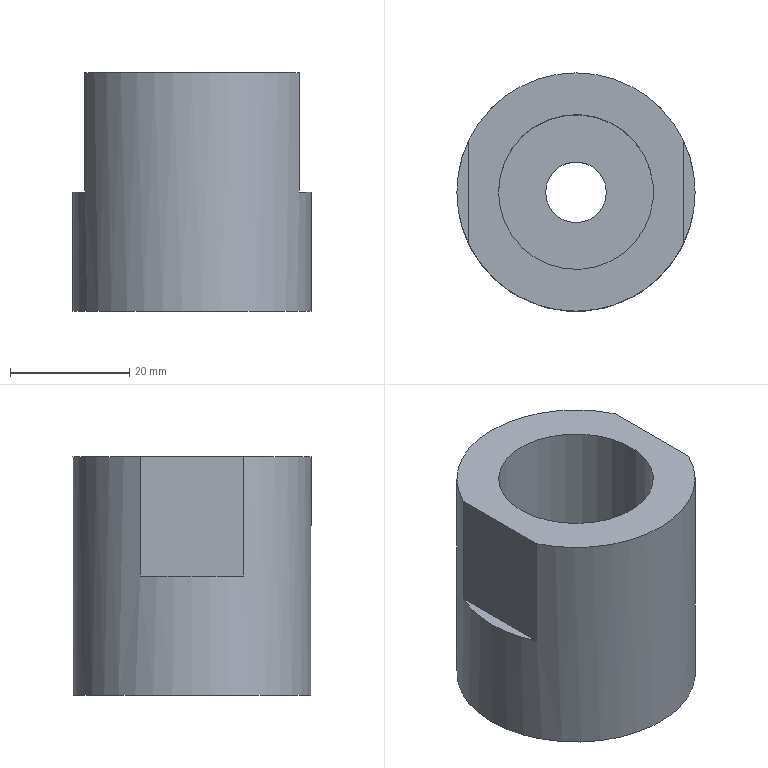Part | NX | features clamp stopper 2 | 1 solid | 10 faces | box 40 x 40 x 40 mm | volume 32581 mm3 | plane 7 | cylinder 3 | commonest cylinder face diameters 10.2 x1 26 x1 40 x1
STEP:
#1=CARTESIAN_POINT('',(-13.,0.,10.));
#2=VERTEX_POINT('',#1);
#3=CARTESIAN_POINT('',(0.,0.,10.));
#4=DIRECTION('',(0.,0.,-1.));
#5=DIRECTION('',(-1.,0.,0.));
#6=AXIS2_PLACEMENT_3D('',#3,#4,#5);
#7=CIRCLE('',#6,13.);
#8=EDGE_CURVE('',#2,#2,#7,.F.);
#9=ORIENTED_EDGE('',*,*,#8,.T.);
#10=EDGE_LOOP('',(#9));
#11=FACE_BOUND('',#10,.T.);
#12=CARTESIAN_POINT('',(5.1,0.,10.));
#13=VERTEX_POINT('',#12);
#14=CARTESIAN_POINT('',(0.,0.,10.));
#15=DIRECTION('',(0.,0.,1.));
#16=DIRECTION('',(1.,0.,0.));
#17=AXIS2_PLACEMENT_3D('',#14,#15,#16);
#18=CIRCLE('',#17,5.1);
#19=EDGE_CURVE('',#13,#13,#18,.F.);
#20=ORIENTED_EDGE('',*,*,#19,.T.);
#21=EDGE_LOOP('',(#20));
#22=FACE_BOUND('',#21,.T.);
#23=CARTESIAN_POINT('',(0.,0.,10.));
#24=DIRECTION('',(0.,0.,-1.));
#25=DIRECTION('',(-1.,0.,0.));
#26=AXIS2_PLACEMENT_3D('',#23,#24,#25);
#27=PLANE('',#26);
#28=ADVANCED_FACE('',(#11,#22),#27,.F.);
#29=ORIENTED_EDGE('',*,*,#8,.F.);
#30=EDGE_LOOP('',(#29));
#31=FACE_BOUND('',#30,.T.);
#32=CARTESIAN_POINT('',(-13.,0.,40.));
#33=VERTEX_POINT('',#32);
#34=CARTESIAN_POINT('',(0.,0.,40.));
#35=DIRECTION('',(0.,0.,-1.));
#36=DIRECTION('',(-1.,0.,0.));
#37=AXIS2_PLACEMENT_3D('',#34,#35,#36);
#38=CIRCLE('',#37,13.);
#39=EDGE_CURVE('',#33,#33,#38,.T.);
#40=ORIENTED_EDGE('',*,*,#39,.F.);
#41=EDGE_LOOP('',(#40));
#42=FACE_BOUND('',#41,.T.);
#43=CARTESIAN_POINT('',(0.,0.,40.));
#44=DIRECTION('',(0.,0.,-1.));
#45=DIRECTION('',(-1.,0.,0.));
#46=AXIS2_PLACEMENT_3D('',#43,#44,#45);
#47=CYLINDRICAL_SURFACE('',#46,13.);
#48=ADVANCED_FACE('',(#31,#42),#47,.F.);
#49=CARTESIAN_POINT('',(5.1,0.,0.));
#50=VERTEX_POINT('',#49);
#51=CARTESIAN_POINT('',(0.,0.,0.));
#52=DIRECTION('',(0.,0.,1.));
#53=DIRECTION('',(1.,0.,0.));
#54=AXIS2_PLACEMENT_3D('',#51,#52,#53);
#55=CIRCLE('',#54,5.1);
#56=EDGE_CURVE('',#50,#50,#55,.F.);
#57=ORIENTED_EDGE('',*,*,#56,.T.);
#58=EDGE_LOOP('',(#57));
#59=FACE_BOUND('',#58,.T.);
#60=ORIENTED_EDGE('',*,*,#19,.F.);
#61=EDGE_LOOP('',(#60));
#62=FACE_BOUND('',#61,.T.);
#63=CARTESIAN_POINT('',(0.,0.,10.));
#64=DIRECTION('',(0.,0.,1.));
#65=DIRECTION('',(1.,0.,0.));
#66=AXIS2_PLACEMENT_3D('',#63,#64,#65);
#67=CYLINDRICAL_SURFACE('',#66,5.1);
#68=ADVANCED_FACE('',(#59,#62),#67,.F.);
#69=CARTESIAN_POINT('',(18.,8.718,20.));
#70=VERTEX_POINT('',#69);
#71=CARTESIAN_POINT('',(18.,-8.718,20.));
#72=VERTEX_POINT('',#71);
#73=CARTESIAN_POINT('',(0.,0.,20.));
#74=DIRECTION('',(0.,0.,-1.));
#75=DIRECTION('',(-1.,0.,0.));
#76=AXIS2_PLACEMENT_3D('',#73,#74,#75);
#77=CIRCLE('',#76,20.);
#78=EDGE_CURVE('',#70,#72,#77,.T.);
#79=ORIENTED_EDGE('',*,*,#78,.F.);
#80=CARTESIAN_POINT('',(18.,-20.,20.));
#81=DIRECTION('',(0.,1.,0.));
#82=VECTOR('',#81,1000.);
#83=LINE('',#80,#82);
#84=EDGE_CURVE('',#72,#70,#83,.T.);
#85=ORIENTED_EDGE('',*,*,#84,.F.);
#86=EDGE_LOOP('',(#79,#85));
#87=FACE_BOUND('',#86,.T.);
#88=CARTESIAN_POINT('',(0.,0.,20.));
#89=DIRECTION('',(0.,0.,1.));
#90=DIRECTION('',(1.,0.,0.));
#91=AXIS2_PLACEMENT_3D('',#88,#89,#90);
#92=PLANE('',#91);
#93=ADVANCED_FACE('',(#87),#92,.T.);
#94=CARTESIAN_POINT('',(18.,8.718,40.));
#95=VERTEX_POINT('',#94);
#96=CARTESIAN_POINT('',(18.,8.718,40.));
#97=DIRECTION('',(0.,0.,-1.));
#98=VECTOR('',#97,1000.);
#99=LINE('',#96,#98);
#100=EDGE_CURVE('',#95,#70,#99,.T.);
#101=ORIENTED_EDGE('',*,*,#100,.F.);
#102=CARTESIAN_POINT('',(18.,-8.718,40.));
#103=VERTEX_POINT('',#102);
#104=CARTESIAN_POINT('',(18.,0.,40.));
#105=DIRECTION('',(0.,1.,0.));
#106=VECTOR('',#105,1000.);
#107=LINE('',#104,#106);
#108=EDGE_CURVE('',#103,#95,#107,.T.);
#109=ORIENTED_EDGE('',*,*,#108,.F.);
#110=CARTESIAN_POINT('',(18.,-8.718,40.));
#111=DIRECTION('',(0.,0.,-1.));
#112=VECTOR('',#111,1000.);
#113=LINE('',#110,#112);
#114=EDGE_CURVE('',#72,#103,#113,.F.);
#115=ORIENTED_EDGE('',*,*,#114,.F.);
#116=ORIENTED_EDGE('',*,*,#84,.T.);
#117=EDGE_LOOP('',(#101,#109,#115,#116));
#118=FACE_BOUND('',#117,.T.);
#119=CARTESIAN_POINT('',(18.,-20.,20.));
#120=DIRECTION('',(1.,0.,0.));
#121=DIRECTION('',(0.,0.,-1.));
#122=AXIS2_PLACEMENT_3D('',#119,#120,#121);
#123=PLANE('',#122);
#124=ADVANCED_FACE('',(#118),#123,.T.);
#125=CARTESIAN_POINT('',(-18.,8.718,40.));
#126=VERTEX_POINT('',#125);
#127=CARTESIAN_POINT('',(0.,0.,40.));
#128=DIRECTION('',(0.,0.,-1.));
#129=DIRECTION('',(-1.,0.,0.));
#130=AXIS2_PLACEMENT_3D('',#127,#128,#129);
#131=CIRCLE('',#130,20.);
#132=EDGE_CURVE('',#126,#95,#131,.T.);
#133=ORIENTED_EDGE('',*,*,#132,.F.);
#134=CARTESIAN_POINT('',(-18.,-8.718,40.));
#135=VERTEX_POINT('',#134);
#136=CARTESIAN_POINT('',(-18.,-20.,40.));
#137=DIRECTION('',(0.,1.,0.));
#138=VECTOR('',#137,1000.);
#139=LINE('',#136,#138);
#140=EDGE_CURVE('',#135,#126,#139,.T.);
#141=ORIENTED_EDGE('',*,*,#140,.F.);
#142=CARTESIAN_POINT('',(0.,0.,40.));
#143=DIRECTION('',(0.,0.,-1.));
#144=DIRECTION('',(-1.,0.,0.));
#145=AXIS2_PLACEMENT_3D('',#142,#143,#144);
#146=CIRCLE('',#145,20.);
#147=EDGE_CURVE('',#103,#135,#146,.T.);
#148=ORIENTED_EDGE('',*,*,#147,.F.);
#149=ORIENTED_EDGE('',*,*,#108,.T.);
#150=EDGE_LOOP('',(#133,#141,#148,#149));
#151=FACE_BOUND('',#150,.T.);
#152=ORIENTED_EDGE('',*,*,#39,.T.);
#153=EDGE_LOOP('',(#152));
#154=FACE_BOUND('',#153,.T.);
#155=CARTESIAN_POINT('',(0.,0.,40.));
#156=DIRECTION('',(0.,0.,1.));
#157=DIRECTION('',(1.,0.,0.));
#158=AXIS2_PLACEMENT_3D('',#155,#156,#157);
#159=PLANE('',#158);
#160=ADVANCED_FACE('',(#151,#154),#159,.T.);
#161=CARTESIAN_POINT('',(-18.,-8.718,20.));
#162=VERTEX_POINT('',#161);
#163=CARTESIAN_POINT('',(-18.,-8.718,40.));
#164=DIRECTION('',(0.,0.,-1.));
#165=VECTOR('',#164,1000.);
#166=LINE('',#163,#165);
#167=EDGE_CURVE('',#135,#162,#166,.T.);
#168=ORIENTED_EDGE('',*,*,#167,.F.);
#169=ORIENTED_EDGE('',*,*,#140,.T.);
#170=CARTESIAN_POINT('',(-18.,8.718,20.));
#171=VERTEX_POINT('',#170);
#172=CARTESIAN_POINT('',(-18.,8.718,40.));
#173=DIRECTION('',(0.,0.,-1.));
#174=VECTOR('',#173,1000.);
#175=LINE('',#172,#174);
#176=EDGE_CURVE('',#171,#126,#175,.F.);
#177=ORIENTED_EDGE('',*,*,#176,.F.);
#178=CARTESIAN_POINT('',(-18.,0.,20.));
#179=DIRECTION('',(0.,1.,0.));
#180=VECTOR('',#179,1000.);
#181=LINE('',#178,#180);
#182=EDGE_CURVE('',#162,#171,#181,.T.);
#183=ORIENTED_EDGE('',*,*,#182,.F.);
#184=EDGE_LOOP('',(#168,#169,#177,#183));
#185=FACE_BOUND('',#184,.T.);
#186=CARTESIAN_POINT('',(-18.,-20.,20.));
#187=DIRECTION('',(-1.,0.,0.));
#188=DIRECTION('',(0.,0.,1.));
#189=AXIS2_PLACEMENT_3D('',#186,#187,#188);
#190=PLANE('',#189);
#191=ADVANCED_FACE('',(#185),#190,.T.);
#192=CARTESIAN_POINT('',(0.,0.,20.));
#193=DIRECTION('',(0.,0.,-1.));
#194=DIRECTION('',(-1.,0.,0.));
#195=AXIS2_PLACEMENT_3D('',#192,#193,#194);
#196=CIRCLE('',#195,20.);
#197=EDGE_CURVE('',#162,#171,#196,.T.);
#198=ORIENTED_EDGE('',*,*,#197,.F.);
#199=ORIENTED_EDGE('',*,*,#182,.T.);
#200=EDGE_LOOP('',(#198,#199));
#201=FACE_BOUND('',#200,.T.);
#202=CARTESIAN_POINT('',(0.,0.,20.));
#203=DIRECTION('',(0.,0.,1.));
#204=DIRECTION('',(1.,0.,0.));
#205=AXIS2_PLACEMENT_3D('',#202,#203,#204);
#206=PLANE('',#205);
#207=ADVANCED_FACE('',(#201),#206,.T.);
#208=CARTESIAN_POINT('',(-20.,0.,0.));
#209=VERTEX_POINT('',#208);
#210=CARTESIAN_POINT('',(0.,0.,0.));
#211=DIRECTION('',(0.,0.,-1.));
#212=DIRECTION('',(-1.,0.,0.));
#213=AXIS2_PLACEMENT_3D('',#210,#211,#212);
#214=CIRCLE('',#213,20.);
#215=EDGE_CURVE('',#209,#209,#214,.F.);
#216=ORIENTED_EDGE('',*,*,#215,.F.);
#217=EDGE_LOOP('',(#216));
#218=FACE_BOUND('',#217,.T.);
#219=ORIENTED_EDGE('',*,*,#56,.F.);
#220=EDGE_LOOP('',(#219));
#221=FACE_BOUND('',#220,.T.);
#222=CARTESIAN_POINT('',(0.,0.,0.));
#223=DIRECTION('',(0.,0.,1.));
#224=DIRECTION('',(1.,0.,0.));
#225=AXIS2_PLACEMENT_3D('',#222,#223,#224);
#226=PLANE('',#225);
#227=ADVANCED_FACE('',(#218,#221),#226,.F.);
#228=ORIENTED_EDGE('',*,*,#100,.T.);
#229=ORIENTED_EDGE('',*,*,#78,.T.);
#230=ORIENTED_EDGE('',*,*,#114,.T.);
#231=ORIENTED_EDGE('',*,*,#147,.T.);
#232=ORIENTED_EDGE('',*,*,#167,.T.);
#233=ORIENTED_EDGE('',*,*,#197,.T.);
#234=ORIENTED_EDGE('',*,*,#176,.T.);
#235=ORIENTED_EDGE('',*,*,#132,.T.);
#236=EDGE_LOOP('',(#228,#229,#230,#231,#232,#233,#234,#235));
#237=FACE_BOUND('',#236,.T.);
#238=ORIENTED_EDGE('',*,*,#215,.T.);
#239=EDGE_LOOP('',(#238));
#240=FACE_BOUND('',#239,.T.);
#241=CARTESIAN_POINT('',(0.,0.,40.));
#242=DIRECTION('',(0.,0.,-1.));
#243=DIRECTION('',(-1.,0.,0.));
#244=AXIS2_PLACEMENT_3D('',#241,#242,#243);
#245=CYLINDRICAL_SURFACE('',#244,20.);
#246=ADVANCED_FACE('',(#237,#240),#245,.T.);
#247=CLOSED_SHELL('',(#28,#48,#68,#93,#124,#160,#191,#207,#227,#246));
#248=MANIFOLD_SOLID_BREP('',#247);
#249=(LENGTH_UNIT()NAMED_UNIT(*)SI_UNIT(.MILLI.,.METRE.));
#250=UNCERTAINTY_MEASURE_WITH_UNIT(LENGTH_MEASURE(0.00001),#249,'','');
#251=(NAMED_UNIT(*)PLANE_ANGLE_UNIT()SI_UNIT($,.RADIAN.));
#252=(NAMED_UNIT(*)SI_UNIT($,.STERADIAN.)SOLID_ANGLE_UNIT());
#253=(GEOMETRIC_REPRESENTATION_CONTEXT(3)GLOBAL_UNCERTAINTY_ASSIGNED_CONTEXT((#250))GLOBAL_UNIT_ASSIGNED_CONTEXT((#249,#251,#252))REPRESENTATION_CONTEXT('',''));
#254=ADVANCED_BREP_SHAPE_REPRESENTATION('',(#248),#253);